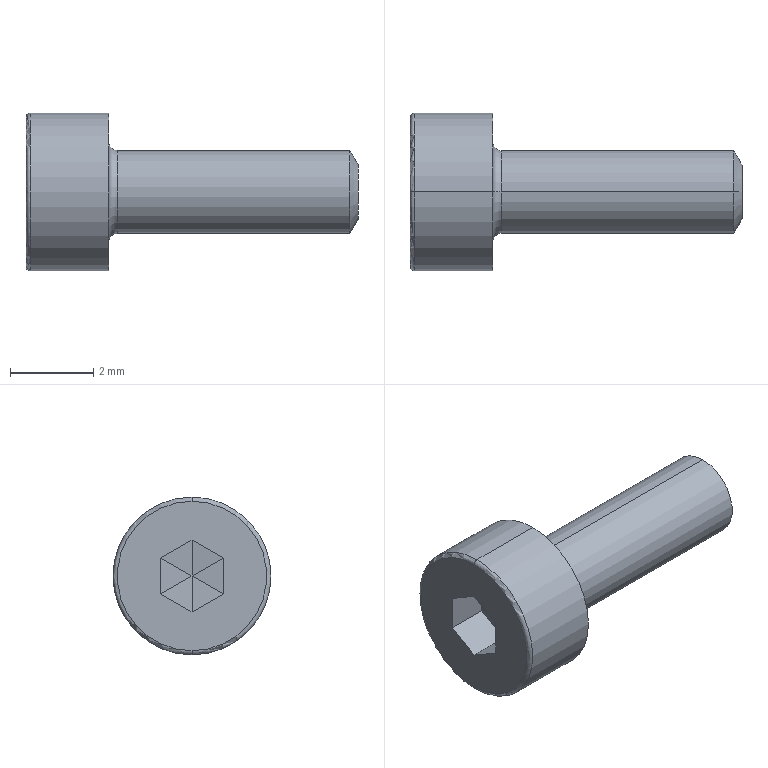Part | SolidWorks | features BlendCut 1, Cut 1, Fillet 1, LPattern 1, RevCut 1, Revolution 1 | 1 solid | 25 faces | box 8 x 3.8 x 3.8 mm | volume 39.383 mm3 | plane 15 | torus 4 | cylinder 4 | cone 2 | commonest cylinder face diameters 2 x2 3.8 x2
STEP:
#1=CARTESIAN_POINT('',(0.,0.,1.8));
#2=VERTEX_POINT('',#1);
#3=CARTESIAN_POINT('',(0.,0.,-1.8));
#4=VERTEX_POINT('',#3);
#5=CARTESIAN_POINT('',(0.,0.,0.));
#6=DIRECTION('',(-1.,0.,0.));
#7=DIRECTION('',(0.,0.,-1.));
#8=AXIS2_PLACEMENT_3D('',#5,#6,#7);
#9=CIRCLE('',#8,1.8);
#10=EDGE_CURVE('',#2,#4,#9,.T.);
#11=ORIENTED_EDGE('',*,*,#10,.F.);
#12=CARTESIAN_POINT('',(0.1,0.,1.9));
#13=VERTEX_POINT('',#12);
#14=CARTESIAN_POINT('',(0.1,0.,1.8));
#15=DIRECTION('',(0.,1.,0.));
#16=DIRECTION('',(0.,0.,1.));
#17=AXIS2_PLACEMENT_3D('',#14,#15,#16);
#18=CIRCLE('',#17,0.1);
#19=EDGE_CURVE('',#2,#13,#18,.T.);
#20=ORIENTED_EDGE('',*,*,#19,.T.);
#21=CARTESIAN_POINT('',(0.1,0.,-1.9));
#22=VERTEX_POINT('',#21);
#23=CARTESIAN_POINT('',(0.1,0.,0.));
#24=DIRECTION('',(1.,0.,0.));
#25=DIRECTION('',(0.,0.,-1.));
#26=AXIS2_PLACEMENT_3D('',#23,#24,#25);
#27=CIRCLE('',#26,1.9);
#28=EDGE_CURVE('',#22,#13,#27,.T.);
#29=ORIENTED_EDGE('',*,*,#28,.F.);
#30=CARTESIAN_POINT('',(0.1,0.,-1.8));
#31=DIRECTION('',(0.,-1.,0.));
#32=DIRECTION('',(0.,0.,-1.));
#33=AXIS2_PLACEMENT_3D('',#30,#31,#32);
#34=CIRCLE('',#33,0.1);
#35=EDGE_CURVE('',#4,#22,#34,.T.);
#36=ORIENTED_EDGE('',*,*,#35,.F.);
#37=EDGE_LOOP('',(#11,#20,#29,#36));
#38=FACE_OUTER_BOUND('',#37,.T.);
#39=CARTESIAN_POINT('',(0.1,0.,0.));
#40=DIRECTION('',(1.,0.,0.));
#41=DIRECTION('',(0.,0.,-1.));
#42=AXIS2_PLACEMENT_3D('',#39,#40,#41);
#43=TOROIDAL_SURFACE('',#42,1.8,0.1);
#44=ADVANCED_FACE('',(#38),#43,.T.);
#45=CARTESIAN_POINT('',(8.,0.,0.6536));
#46=VERTEX_POINT('',#45);
#47=CARTESIAN_POINT('',(8.,0.,-0.6536));
#48=VERTEX_POINT('',#47);
#49=CARTESIAN_POINT('',(8.,0.,0.));
#50=DIRECTION('',(-1.,0.,0.));
#51=DIRECTION('',(0.,0.,1.));
#52=AXIS2_PLACEMENT_3D('',#49,#50,#51);
#53=CIRCLE('',#52,0.6536);
#54=EDGE_CURVE('',#46,#48,#53,.T.);
#55=ORIENTED_EDGE('',*,*,#54,.T.);
#56=CARTESIAN_POINT('',(7.8,0.,-1.));
#57=VERTEX_POINT('',#56);
#58=CARTESIAN_POINT('',(7.8,0.,-1.));
#59=DIRECTION('',(-0.5,0.,-0.866));
#60=VECTOR('',#59,1000.);
#61=LINE('',#58,#60);
#62=EDGE_CURVE('',#48,#57,#61,.T.);
#63=ORIENTED_EDGE('',*,*,#62,.T.);
#64=CARTESIAN_POINT('',(7.8,0.,1.));
#65=VERTEX_POINT('',#64);
#66=CARTESIAN_POINT('',(7.8,0.,0.));
#67=DIRECTION('',(-1.,0.,0.));
#68=DIRECTION('',(0.,0.,1.));
#69=AXIS2_PLACEMENT_3D('',#66,#67,#68);
#70=CIRCLE('',#69,1.);
#71=EDGE_CURVE('',#65,#57,#70,.T.);
#72=ORIENTED_EDGE('',*,*,#71,.F.);
#73=CARTESIAN_POINT('',(7.8,0.,1.));
#74=DIRECTION('',(-0.5,0.,0.866));
#75=VECTOR('',#74,1000.);
#76=LINE('',#73,#75);
#77=EDGE_CURVE('',#46,#65,#76,.T.);
#78=ORIENTED_EDGE('',*,*,#77,.F.);
#79=EDGE_LOOP('',(#55,#63,#72,#78));
#80=FACE_OUTER_BOUND('',#79,.T.);
#81=CARTESIAN_POINT('',(7.8,0.,0.));
#82=DIRECTION('',(-1.,0.,0.));
#83=DIRECTION('',(0.,0.,1.));
#84=AXIS2_PLACEMENT_3D('',#81,#82,#83);
#85=CONICAL_SURFACE('',#84,1.,1.047);
#86=ADVANCED_FACE('',(#80),#85,.T.);
#87=CARTESIAN_POINT('',(2.,0.,-1.2));
#88=VERTEX_POINT('',#87);
#89=CARTESIAN_POINT('',(2.,0.,1.2));
#90=VERTEX_POINT('',#89);
#91=CARTESIAN_POINT('',(2.,0.,0.));
#92=DIRECTION('',(-1.,0.,0.));
#93=DIRECTION('',(0.,0.,1.));
#94=AXIS2_PLACEMENT_3D('',#91,#92,#93);
#95=CIRCLE('',#94,1.2);
#96=EDGE_CURVE('',#88,#90,#95,.T.);
#97=ORIENTED_EDGE('',*,*,#96,.F.);
#98=CARTESIAN_POINT('',(2.2,0.,-1.));
#99=VERTEX_POINT('',#98);
#100=CARTESIAN_POINT('',(2.2,0.,-1.2));
#101=DIRECTION('',(0.,1.,0.));
#102=DIRECTION('',(0.,0.,1.));
#103=AXIS2_PLACEMENT_3D('',#100,#101,#102);
#104=CIRCLE('',#103,0.2);
#105=EDGE_CURVE('',#88,#99,#104,.T.);
#106=ORIENTED_EDGE('',*,*,#105,.T.);
#107=CARTESIAN_POINT('',(2.2,0.,1.));
#108=VERTEX_POINT('',#107);
#109=CARTESIAN_POINT('',(2.2,0.,0.));
#110=DIRECTION('',(-1.,0.,0.));
#111=DIRECTION('',(0.,0.,1.));
#112=AXIS2_PLACEMENT_3D('',#109,#110,#111);
#113=CIRCLE('',#112,1.);
#114=EDGE_CURVE('',#99,#108,#113,.T.);
#115=ORIENTED_EDGE('',*,*,#114,.T.);
#116=CARTESIAN_POINT('',(2.2,0.,1.2));
#117=DIRECTION('',(0.,-1.,0.));
#118=DIRECTION('',(0.,0.,-1.));
#119=AXIS2_PLACEMENT_3D('',#116,#117,#118);
#120=CIRCLE('',#119,0.2);
#121=EDGE_CURVE('',#90,#108,#120,.T.);
#122=ORIENTED_EDGE('',*,*,#121,.F.);
#123=EDGE_LOOP('',(#97,#106,#115,#122));
#124=FACE_OUTER_BOUND('',#123,.T.);
#125=CARTESIAN_POINT('',(2.2,0.,0.));
#126=DIRECTION('',(-1.,0.,0.));
#127=DIRECTION('',(0.,0.,1.));
#128=AXIS2_PLACEMENT_3D('',#125,#126,#127);
#129=TOROIDAL_SURFACE('',#128,1.2,0.2);
#130=ADVANCED_FACE('',(#124),#129,.F.);
#131=CARTESIAN_POINT('',(2.,0.,1.9));
#132=VERTEX_POINT('',#131);
#133=CARTESIAN_POINT('',(2.,0.,-1.9));
#134=VERTEX_POINT('',#133);
#135=CARTESIAN_POINT('',(2.,0.,0.));
#136=DIRECTION('',(-1.,0.,0.));
#137=DIRECTION('',(0.,0.,1.));
#138=AXIS2_PLACEMENT_3D('',#135,#136,#137);
#139=CIRCLE('',#138,1.9);
#140=EDGE_CURVE('',#132,#134,#139,.T.);
#141=ORIENTED_EDGE('',*,*,#140,.T.);
#142=CARTESIAN_POINT('',(0.,0.,-1.9));
#143=DIRECTION('',(-1.,0.,0.));
#144=VECTOR('',#143,1000.);
#145=LINE('',#142,#144);
#146=EDGE_CURVE('',#134,#22,#145,.T.);
#147=ORIENTED_EDGE('',*,*,#146,.T.);
#148=ORIENTED_EDGE('',*,*,#28,.T.);
#149=CARTESIAN_POINT('',(0.,0.,1.9));
#150=DIRECTION('',(-1.,0.,0.));
#151=VECTOR('',#150,1000.);
#152=LINE('',#149,#151);
#153=EDGE_CURVE('',#132,#13,#152,.T.);
#154=ORIENTED_EDGE('',*,*,#153,.F.);
#155=EDGE_LOOP('',(#141,#147,#148,#154));
#156=FACE_OUTER_BOUND('',#155,.T.);
#157=CARTESIAN_POINT('',(0.,0.,0.));
#158=DIRECTION('',(-1.,0.,0.));
#159=DIRECTION('',(0.,0.,1.));
#160=AXIS2_PLACEMENT_3D('',#157,#158,#159);
#161=CYLINDRICAL_SURFACE('',#160,1.9);
#162=ADVANCED_FACE('',(#156),#161,.T.);
#163=ORIENTED_EDGE('',*,*,#71,.T.);
#164=CARTESIAN_POINT('',(0.,0.,-1.));
#165=DIRECTION('',(-1.,0.,0.));
#166=VECTOR('',#165,1000.);
#167=LINE('',#164,#166);
#168=EDGE_CURVE('',#57,#99,#167,.T.);
#169=ORIENTED_EDGE('',*,*,#168,.T.);
#170=CARTESIAN_POINT('',(2.2,0.,0.));
#171=DIRECTION('',(-1.,0.,0.));
#172=DIRECTION('',(0.,0.,1.));
#173=AXIS2_PLACEMENT_3D('',#170,#171,#172);
#174=CIRCLE('',#173,1.);
#175=EDGE_CURVE('',#108,#99,#174,.T.);
#176=ORIENTED_EDGE('',*,*,#175,.F.);
#177=CARTESIAN_POINT('',(0.,0.,1.));
#178=DIRECTION('',(-1.,0.,0.));
#179=VECTOR('',#178,1000.);
#180=LINE('',#177,#179);
#181=EDGE_CURVE('',#65,#108,#180,.T.);
#182=ORIENTED_EDGE('',*,*,#181,.F.);
#183=EDGE_LOOP('',(#163,#169,#176,#182));
#184=FACE_OUTER_BOUND('',#183,.T.);
#185=CARTESIAN_POINT('',(0.,0.,0.));
#186=DIRECTION('',(-1.,0.,0.));
#187=DIRECTION('',(0.,0.,1.));
#188=AXIS2_PLACEMENT_3D('',#185,#186,#187);
#189=CYLINDRICAL_SURFACE('',#188,1.);
#190=ADVANCED_FACE('',(#184),#189,.T.);
#191=ORIENTED_EDGE('',*,*,#168,.F.);
#192=CARTESIAN_POINT('',(7.8,0.,0.));
#193=DIRECTION('',(-1.,0.,0.));
#194=DIRECTION('',(0.,0.,1.));
#195=AXIS2_PLACEMENT_3D('',#192,#193,#194);
#196=CIRCLE('',#195,1.);
#197=EDGE_CURVE('',#57,#65,#196,.T.);
#198=ORIENTED_EDGE('',*,*,#197,.T.);
#199=ORIENTED_EDGE('',*,*,#181,.T.);
#200=ORIENTED_EDGE('',*,*,#114,.F.);
#201=EDGE_LOOP('',(#191,#198,#199,#200));
#202=FACE_OUTER_BOUND('',#201,.T.);
#203=CARTESIAN_POINT('',(0.,0.,0.));
#204=DIRECTION('',(-1.,0.,0.));
#205=DIRECTION('',(0.,0.,1.));
#206=AXIS2_PLACEMENT_3D('',#203,#204,#205);
#207=CYLINDRICAL_SURFACE('',#206,1.);
#208=ADVANCED_FACE('',(#202),#207,.T.);
#209=CARTESIAN_POINT('',(0.,0.,0.));
#210=DIRECTION('',(-1.,0.,0.));
#211=DIRECTION('',(0.,0.,-1.));
#212=AXIS2_PLACEMENT_3D('',#209,#210,#211);
#213=CIRCLE('',#212,1.8);
#214=EDGE_CURVE('',#4,#2,#213,.T.);
#215=ORIENTED_EDGE('',*,*,#214,.T.);
#216=ORIENTED_EDGE('',*,*,#10,.T.);
#217=EDGE_LOOP('',(#215,#216));
#218=FACE_OUTER_BOUND('',#217,.T.);
#219=CARTESIAN_POINT('',(0.,0.,0.865));
#220=VERTEX_POINT('',#219);
#221=CARTESIAN_POINT('',(0.,0.7491,0.4325));
#222=VERTEX_POINT('',#221);
#223=CARTESIAN_POINT('',(0.,0.,0.865));
#224=DIRECTION('',(0.,0.866,-0.5));
#225=VECTOR('',#224,1000.);
#226=LINE('',#223,#225);
#227=EDGE_CURVE('',#220,#222,#226,.T.);
#228=ORIENTED_EDGE('',*,*,#227,.F.);
#229=CARTESIAN_POINT('',(0.,-0.7491,0.4325));
#230=VERTEX_POINT('',#229);
#231=CARTESIAN_POINT('',(0.,-0.7491,0.4325));
#232=DIRECTION('',(0.,0.866,0.5));
#233=VECTOR('',#232,1000.);
#234=LINE('',#231,#233);
#235=EDGE_CURVE('',#230,#220,#234,.T.);
#236=ORIENTED_EDGE('',*,*,#235,.F.);
#237=CARTESIAN_POINT('',(0.,-0.7491,-0.4325));
#238=VERTEX_POINT('',#237);
#239=CARTESIAN_POINT('',(0.,-0.7491,-0.4325));
#240=DIRECTION('',(0.,0.,1.));
#241=VECTOR('',#240,1000.);
#242=LINE('',#239,#241);
#243=EDGE_CURVE('',#238,#230,#242,.T.);
#244=ORIENTED_EDGE('',*,*,#243,.F.);
#245=CARTESIAN_POINT('',(0.,0.,-0.865));
#246=VERTEX_POINT('',#245);
#247=CARTESIAN_POINT('',(0.,0.,-0.865));
#248=DIRECTION('',(0.,-0.866,0.5));
#249=VECTOR('',#248,1000.);
#250=LINE('',#247,#249);
#251=EDGE_CURVE('',#246,#238,#250,.T.);
#252=ORIENTED_EDGE('',*,*,#251,.F.);
#253=CARTESIAN_POINT('',(0.,0.7491,-0.4325));
#254=VERTEX_POINT('',#253);
#255=CARTESIAN_POINT('',(0.,0.7491,-0.4325));
#256=DIRECTION('',(0.,-0.866,-0.5));
#257=VECTOR('',#256,1000.);
#258=LINE('',#255,#257);
#259=EDGE_CURVE('',#254,#246,#258,.T.);
#260=ORIENTED_EDGE('',*,*,#259,.F.);
#261=CARTESIAN_POINT('',(0.,0.7491,0.4325));
#262=DIRECTION('',(0.,0.,-1.));
#263=VECTOR('',#262,1000.);
#264=LINE('',#261,#263);
#265=EDGE_CURVE('',#222,#254,#264,.T.);
#266=ORIENTED_EDGE('',*,*,#265,.F.);
#267=EDGE_LOOP('',(#228,#236,#244,#252,#260,#266));
#268=FACE_BOUND('',#267,.T.);
#269=CARTESIAN_POINT('',(0.,0.,0.));
#270=DIRECTION('',(1.,0.,0.));
#271=DIRECTION('',(0.,0.,-1.));
#272=AXIS2_PLACEMENT_3D('',#269,#270,#271);
#273=PLANE('',#272);
#274=ADVANCED_FACE('',(#218,#268),#273,.F.);
#275=ORIENTED_EDGE('',*,*,#146,.F.);
#276=CARTESIAN_POINT('',(2.,0.,0.));
#277=DIRECTION('',(-1.,0.,0.));
#278=DIRECTION('',(0.,0.,1.));
#279=AXIS2_PLACEMENT_3D('',#276,#277,#278);
#280=CIRCLE('',#279,1.9);
#281=EDGE_CURVE('',#134,#132,#280,.T.);
#282=ORIENTED_EDGE('',*,*,#281,.T.);
#283=ORIENTED_EDGE('',*,*,#153,.T.);
#284=CARTESIAN_POINT('',(0.1,0.,0.));
#285=DIRECTION('',(1.,0.,0.));
#286=DIRECTION('',(0.,0.,-1.));
#287=AXIS2_PLACEMENT_3D('',#284,#285,#286);
#288=CIRCLE('',#287,1.9);
#289=EDGE_CURVE('',#13,#22,#288,.T.);
#290=ORIENTED_EDGE('',*,*,#289,.T.);
#291=EDGE_LOOP('',(#275,#282,#283,#290));
#292=FACE_OUTER_BOUND('',#291,.T.);
#293=CARTESIAN_POINT('',(0.,0.,0.));
#294=DIRECTION('',(-1.,0.,0.));
#295=DIRECTION('',(0.,0.,1.));
#296=AXIS2_PLACEMENT_3D('',#293,#294,#295);
#297=CYLINDRICAL_SURFACE('',#296,1.9);
#298=ADVANCED_FACE('',(#292),#297,.T.);
#299=ORIENTED_EDGE('',*,*,#140,.F.);
#300=ORIENTED_EDGE('',*,*,#281,.F.);
#301=EDGE_LOOP('',(#299,#300));
#302=FACE_OUTER_BOUND('',#301,.T.);
#303=CARTESIAN_POINT('',(2.,0.,0.));
#304=DIRECTION('',(-1.,0.,0.));
#305=DIRECTION('',(0.,0.,1.));
#306=AXIS2_PLACEMENT_3D('',#303,#304,#305);
#307=CIRCLE('',#306,1.2);
#308=EDGE_CURVE('',#90,#88,#307,.T.);
#309=ORIENTED_EDGE('',*,*,#308,.T.);
#310=ORIENTED_EDGE('',*,*,#96,.T.);
#311=EDGE_LOOP('',(#309,#310));
#312=FACE_BOUND('',#311,.T.);
#313=CARTESIAN_POINT('',(2.,1.9,0.));
#314=DIRECTION('',(-1.,0.,0.));
#315=DIRECTION('',(0.,0.,1.));
#316=AXIS2_PLACEMENT_3D('',#313,#314,#315);
#317=PLANE('',#316);
#318=ADVANCED_FACE('',(#302,#312),#317,.F.);
#319=ORIENTED_EDGE('',*,*,#105,.F.);
#320=ORIENTED_EDGE('',*,*,#308,.F.);
#321=ORIENTED_EDGE('',*,*,#121,.T.);
#322=ORIENTED_EDGE('',*,*,#175,.T.);
#323=EDGE_LOOP('',(#319,#320,#321,#322));
#324=FACE_OUTER_BOUND('',#323,.T.);
#325=CARTESIAN_POINT('',(2.2,0.,0.));
#326=DIRECTION('',(-1.,0.,0.));
#327=DIRECTION('',(0.,0.,1.));
#328=AXIS2_PLACEMENT_3D('',#325,#326,#327);
#329=TOROIDAL_SURFACE('',#328,1.2,0.2);
#330=ADVANCED_FACE('',(#324),#329,.F.);
#331=ORIENTED_EDGE('',*,*,#235,.T.);
#332=CARTESIAN_POINT('',(1.,0.,0.865));
#333=VERTEX_POINT('',#332);
#334=CARTESIAN_POINT('',(1.,0.,0.865));
#335=DIRECTION('',(-1.,0.,0.));
#336=VECTOR('',#335,1000.);
#337=LINE('',#334,#336);
#338=EDGE_CURVE('',#333,#220,#337,.T.);
#339=ORIENTED_EDGE('',*,*,#338,.F.);
#340=CARTESIAN_POINT('',(1.,-0.7491,0.4325));
#341=VERTEX_POINT('',#340);
#342=CARTESIAN_POINT('',(1.,-0.7491,0.4325));
#343=DIRECTION('',(0.,0.866,0.5));
#344=VECTOR('',#343,1000.);
#345=LINE('',#342,#344);
#346=EDGE_CURVE('',#341,#333,#345,.T.);
#347=ORIENTED_EDGE('',*,*,#346,.F.);
#348=CARTESIAN_POINT('',(1.,-0.7491,0.4325));
#349=DIRECTION('',(-1.,0.,0.));
#350=VECTOR('',#349,1000.);
#351=LINE('',#348,#350);
#352=EDGE_CURVE('',#341,#230,#351,.T.);
#353=ORIENTED_EDGE('',*,*,#352,.T.);
#354=EDGE_LOOP('',(#331,#339,#347,#353));
#355=FACE_OUTER_BOUND('',#354,.T.);
#356=CARTESIAN_POINT('',(1.,-0.7491,0.4325));
#357=DIRECTION('',(0.,-0.5,0.866));
#358=DIRECTION('',(0.,-0.866,-0.5));
#359=AXIS2_PLACEMENT_3D('',#356,#357,#358);
#360=PLANE('',#359);
#361=ADVANCED_FACE('',(#355),#360,.F.);
#362=ORIENTED_EDGE('',*,*,#243,.T.);
#363=ORIENTED_EDGE('',*,*,#352,.F.);
#364=CARTESIAN_POINT('',(1.,-0.7491,-0.4325));
#365=VERTEX_POINT('',#364);
#366=CARTESIAN_POINT('',(1.,-0.7491,-0.4325));
#367=DIRECTION('',(0.,0.,1.));
#368=VECTOR('',#367,1000.);
#369=LINE('',#366,#368);
#370=EDGE_CURVE('',#365,#341,#369,.T.);
#371=ORIENTED_EDGE('',*,*,#370,.F.);
#372=CARTESIAN_POINT('',(1.,-0.7491,-0.4325));
#373=DIRECTION('',(-1.,0.,0.));
#374=VECTOR('',#373,1000.);
#375=LINE('',#372,#374);
#376=EDGE_CURVE('',#365,#238,#375,.T.);
#377=ORIENTED_EDGE('',*,*,#376,.T.);
#378=EDGE_LOOP('',(#362,#363,#371,#377));
#379=FACE_OUTER_BOUND('',#378,.T.);
#380=CARTESIAN_POINT('',(1.,-0.7491,-0.4325));
#381=DIRECTION('',(0.,-1.,0.));
#382=DIRECTION('',(0.,0.,-1.));
#383=AXIS2_PLACEMENT_3D('',#380,#381,#382);
#384=PLANE('',#383);
#385=ADVANCED_FACE('',(#379),#384,.F.);
#386=ORIENTED_EDGE('',*,*,#251,.T.);
#387=ORIENTED_EDGE('',*,*,#376,.F.);
#388=CARTESIAN_POINT('',(1.,0.,-0.865));
#389=VERTEX_POINT('',#388);
#390=CARTESIAN_POINT('',(1.,0.,-0.865));
#391=DIRECTION('',(0.,-0.866,0.5));
#392=VECTOR('',#391,1000.);
#393=LINE('',#390,#392);
#394=EDGE_CURVE('',#389,#365,#393,.T.);
#395=ORIENTED_EDGE('',*,*,#394,.F.);
#396=CARTESIAN_POINT('',(1.,0.,-0.865));
#397=DIRECTION('',(-1.,0.,0.));
#398=VECTOR('',#397,1000.);
#399=LINE('',#396,#398);
#400=EDGE_CURVE('',#389,#246,#399,.T.);
#401=ORIENTED_EDGE('',*,*,#400,.T.);
#402=EDGE_LOOP('',(#386,#387,#395,#401));
#403=FACE_OUTER_BOUND('',#402,.T.);
#404=CARTESIAN_POINT('',(1.,0.,-0.865));
#405=DIRECTION('',(0.,-0.5,-0.866));
#406=DIRECTION('',(0.,0.866,-0.5));
#407=AXIS2_PLACEMENT_3D('',#404,#405,#406);
#408=PLANE('',#407);
#409=ADVANCED_FACE('',(#403),#408,.F.);
#410=ORIENTED_EDGE('',*,*,#259,.T.);
#411=ORIENTED_EDGE('',*,*,#400,.F.);
#412=CARTESIAN_POINT('',(1.,0.7491,-0.4325));
#413=VERTEX_POINT('',#412);
#414=CARTESIAN_POINT('',(1.,0.7491,-0.4325));
#415=DIRECTION('',(0.,-0.866,-0.5));
#416=VECTOR('',#415,1000.);
#417=LINE('',#414,#416);
#418=EDGE_CURVE('',#413,#389,#417,.T.);
#419=ORIENTED_EDGE('',*,*,#418,.F.);
#420=CARTESIAN_POINT('',(1.,0.7491,-0.4325));
#421=DIRECTION('',(-1.,0.,0.));
#422=VECTOR('',#421,1000.);
#423=LINE('',#420,#422);
#424=EDGE_CURVE('',#413,#254,#423,.T.);
#425=ORIENTED_EDGE('',*,*,#424,.T.);
#426=EDGE_LOOP('',(#410,#411,#419,#425));
#427=FACE_OUTER_BOUND('',#426,.T.);
#428=CARTESIAN_POINT('',(1.,0.7491,-0.4325));
#429=DIRECTION('',(0.,0.5,-0.866));
#430=DIRECTION('',(0.,0.866,0.5));
#431=AXIS2_PLACEMENT_3D('',#428,#429,#430);
#432=PLANE('',#431);
#433=ADVANCED_FACE('',(#427),#432,.F.);
#434=ORIENTED_EDGE('',*,*,#265,.T.);
#435=ORIENTED_EDGE('',*,*,#424,.F.);
#436=CARTESIAN_POINT('',(1.,0.7491,0.4325));
#437=VERTEX_POINT('',#436);
#438=CARTESIAN_POINT('',(1.,0.7491,0.4325));
#439=DIRECTION('',(0.,0.,-1.));
#440=VECTOR('',#439,1000.);
#441=LINE('',#438,#440);
#442=EDGE_CURVE('',#437,#413,#441,.T.);
#443=ORIENTED_EDGE('',*,*,#442,.F.);
#444=CARTESIAN_POINT('',(1.,0.7491,0.4325));
#445=DIRECTION('',(-1.,0.,0.));
#446=VECTOR('',#445,1000.);
#447=LINE('',#444,#446);
#448=EDGE_CURVE('',#437,#222,#447,.T.);
#449=ORIENTED_EDGE('',*,*,#448,.T.);
#450=EDGE_LOOP('',(#434,#435,#443,#449));
#451=FACE_OUTER_BOUND('',#450,.T.);
#452=CARTESIAN_POINT('',(1.,0.7491,0.4325));
#453=DIRECTION('',(0.,1.,0.));
#454=DIRECTION('',(0.,0.,1.));
#455=AXIS2_PLACEMENT_3D('',#452,#453,#454);
#456=PLANE('',#455);
#457=ADVANCED_FACE('',(#451),#456,.F.);
#458=ORIENTED_EDGE('',*,*,#227,.T.);
#459=ORIENTED_EDGE('',*,*,#448,.F.);
#460=CARTESIAN_POINT('',(1.,0.,0.865));
#461=DIRECTION('',(0.,0.866,-0.5));
#462=VECTOR('',#461,1000.);
#463=LINE('',#460,#462);
#464=EDGE_CURVE('',#333,#437,#463,.T.);
#465=ORIENTED_EDGE('',*,*,#464,.F.);
#466=ORIENTED_EDGE('',*,*,#338,.T.);
#467=EDGE_LOOP('',(#458,#459,#465,#466));
#468=FACE_OUTER_BOUND('',#467,.T.);
#469=CARTESIAN_POINT('',(1.,0.,0.865));
#470=DIRECTION('',(0.,0.5,0.866));
#471=DIRECTION('',(0.,-0.866,0.5));
#472=AXIS2_PLACEMENT_3D('',#469,#470,#471);
#473=PLANE('',#472);
#474=ADVANCED_FACE('',(#468),#473,.F.);
#475=CARTESIAN_POINT('',(1.067,0.,0.));
#476=VERTEX_POINT('',#475);
#477=CARTESIAN_POINT('',(1.067,0.,0.));
#478=DIRECTION('',(-0.07711,-0.8634,-0.4985));
#479=VECTOR('',#478,1000.);
#480=LINE('',#477,#479);
#481=EDGE_CURVE('',#476,#365,#480,.T.);
#482=ORIENTED_EDGE('',*,*,#481,.F.);
#483=CARTESIAN_POINT('',(1.067,0.,0.));
#484=DIRECTION('',(-0.07711,0.,-0.997));
#485=VECTOR('',#484,1000.);
#486=LINE('',#483,#485);
#487=EDGE_CURVE('',#476,#389,#486,.T.);
#488=ORIENTED_EDGE('',*,*,#487,.T.);
#489=ORIENTED_EDGE('',*,*,#394,.T.);
#490=EDGE_LOOP('',(#482,#488,#489));
#491=FACE_OUTER_BOUND('',#490,.T.);
#492=CARTESIAN_POINT('',(1.,-0.7491,-0.4325));
#493=DIRECTION('',(-0.996,0.04448,0.07704));
#494=DIRECTION('',(0.07711,0.,0.997));
#495=AXIS2_PLACEMENT_3D('',#492,#493,#494);
#496=PLANE('',#495);
#497=ADVANCED_FACE('',(#491),#496,.T.);
#498=ORIENTED_EDGE('',*,*,#487,.F.);
#499=CARTESIAN_POINT('',(1.067,0.,0.));
#500=DIRECTION('',(-0.07711,0.8634,-0.4985));
#501=VECTOR('',#500,1000.);
#502=LINE('',#499,#501);
#503=EDGE_CURVE('',#476,#413,#502,.T.);
#504=ORIENTED_EDGE('',*,*,#503,.T.);
#505=ORIENTED_EDGE('',*,*,#418,.T.);
#506=EDGE_LOOP('',(#498,#504,#505));
#507=FACE_OUTER_BOUND('',#506,.T.);
#508=CARTESIAN_POINT('',(1.,0.,-0.865));
#509=DIRECTION('',(-0.996,-0.04448,0.07704));
#510=DIRECTION('',(0.07711,0.,0.997));
#511=AXIS2_PLACEMENT_3D('',#508,#509,#510);
#512=PLANE('',#511);
#513=ADVANCED_FACE('',(#507),#512,.T.);
#514=CARTESIAN_POINT('',(1.067,0.,0.));
#515=DIRECTION('',(-0.07711,-0.8634,0.4985));
#516=VECTOR('',#515,1000.);
#517=LINE('',#514,#516);
#518=EDGE_CURVE('',#476,#341,#517,.T.);
#519=ORIENTED_EDGE('',*,*,#518,.F.);
#520=ORIENTED_EDGE('',*,*,#481,.T.);
#521=ORIENTED_EDGE('',*,*,#370,.T.);
#522=EDGE_LOOP('',(#519,#520,#521));
#523=FACE_OUTER_BOUND('',#522,.T.);
#524=CARTESIAN_POINT('',(1.,-0.7491,0.4325));
#525=DIRECTION('',(-0.996,0.08895,0.));
#526=DIRECTION('',(-0.08895,-0.996,0.));
#527=AXIS2_PLACEMENT_3D('',#524,#525,#526);
#528=PLANE('',#527);
#529=ADVANCED_FACE('',(#523),#528,.T.);
#530=ORIENTED_EDGE('',*,*,#503,.F.);
#531=CARTESIAN_POINT('',(1.067,0.,0.));
#532=DIRECTION('',(-0.07711,0.8634,0.4985));
#533=VECTOR('',#532,1000.);
#534=LINE('',#531,#533);
#535=EDGE_CURVE('',#476,#437,#534,.T.);
#536=ORIENTED_EDGE('',*,*,#535,.T.);
#537=ORIENTED_EDGE('',*,*,#442,.T.);
#538=EDGE_LOOP('',(#530,#536,#537));
#539=FACE_OUTER_BOUND('',#538,.T.);
#540=CARTESIAN_POINT('',(1.,0.7491,-0.4325));
#541=DIRECTION('',(-0.996,-0.08895,0.));
#542=DIRECTION('',(0.08895,-0.996,0.));
#543=AXIS2_PLACEMENT_3D('',#540,#541,#542);
#544=PLANE('',#543);
#545=ADVANCED_FACE('',(#539),#544,.T.);
#546=CARTESIAN_POINT('',(1.067,0.,0.));
#547=DIRECTION('',(-0.07711,0.,0.997));
#548=VECTOR('',#547,1000.);
#549=LINE('',#546,#548);
#550=EDGE_CURVE('',#476,#333,#549,.T.);
#551=ORIENTED_EDGE('',*,*,#550,.F.);
#552=ORIENTED_EDGE('',*,*,#518,.T.);
#553=ORIENTED_EDGE('',*,*,#346,.T.);
#554=EDGE_LOOP('',(#551,#552,#553));
#555=FACE_OUTER_BOUND('',#554,.T.);
#556=CARTESIAN_POINT('',(1.,0.,0.865));
#557=DIRECTION('',(-0.996,0.04448,-0.07704));
#558=DIRECTION('',(-0.07711,0.,0.997));
#559=AXIS2_PLACEMENT_3D('',#556,#557,#558);
#560=PLANE('',#559);
#561=ADVANCED_FACE('',(#555),#560,.T.);
#562=ORIENTED_EDGE('',*,*,#535,.F.);
#563=ORIENTED_EDGE('',*,*,#550,.T.);
#564=ORIENTED_EDGE('',*,*,#464,.T.);
#565=EDGE_LOOP('',(#562,#563,#564));
#566=FACE_OUTER_BOUND('',#565,.T.);
#567=CARTESIAN_POINT('',(1.,0.7491,0.4325));
#568=DIRECTION('',(-0.996,-0.04448,-0.07704));
#569=DIRECTION('',(-0.07711,0.,0.997));
#570=AXIS2_PLACEMENT_3D('',#567,#568,#569);
#571=PLANE('',#570);
#572=ADVANCED_FACE('',(#566),#571,.T.);
#573=ORIENTED_EDGE('',*,*,#62,.F.);
#574=CARTESIAN_POINT('',(8.,0.,0.));
#575=DIRECTION('',(-1.,0.,0.));
#576=DIRECTION('',(0.,0.,1.));
#577=AXIS2_PLACEMENT_3D('',#574,#575,#576);
#578=CIRCLE('',#577,0.6536);
#579=EDGE_CURVE('',#48,#46,#578,.T.);
#580=ORIENTED_EDGE('',*,*,#579,.T.);
#581=ORIENTED_EDGE('',*,*,#77,.T.);
#582=ORIENTED_EDGE('',*,*,#197,.F.);
#583=EDGE_LOOP('',(#573,#580,#581,#582));
#584=FACE_OUTER_BOUND('',#583,.T.);
#585=CARTESIAN_POINT('',(7.8,0.,0.));
#586=DIRECTION('',(-1.,0.,0.));
#587=DIRECTION('',(0.,0.,1.));
#588=AXIS2_PLACEMENT_3D('',#585,#586,#587);
#589=CONICAL_SURFACE('',#588,1.,1.047);
#590=ADVANCED_FACE('',(#584),#589,.T.);
#591=ORIENTED_EDGE('',*,*,#54,.F.);
#592=ORIENTED_EDGE('',*,*,#579,.F.);
#593=EDGE_LOOP('',(#591,#592));
#594=FACE_OUTER_BOUND('',#593,.T.);
#595=CARTESIAN_POINT('',(8.,1.,0.));
#596=DIRECTION('',(-1.,0.,0.));
#597=DIRECTION('',(0.,0.,1.));
#598=AXIS2_PLACEMENT_3D('',#595,#596,#597);
#599=PLANE('',#598);
#600=ADVANCED_FACE('',(#594),#599,.F.);
#601=ORIENTED_EDGE('',*,*,#19,.F.);
#602=ORIENTED_EDGE('',*,*,#214,.F.);
#603=ORIENTED_EDGE('',*,*,#35,.T.);
#604=ORIENTED_EDGE('',*,*,#289,.F.);
#605=EDGE_LOOP('',(#601,#602,#603,#604));
#606=FACE_OUTER_BOUND('',#605,.T.);
#607=CARTESIAN_POINT('',(0.1,0.,0.));
#608=DIRECTION('',(1.,0.,0.));
#609=DIRECTION('',(0.,0.,-1.));
#610=AXIS2_PLACEMENT_3D('',#607,#608,#609);
#611=TOROIDAL_SURFACE('',#610,1.8,0.1);
#612=ADVANCED_FACE('',(#606),#611,.T.);
#613=CLOSED_SHELL('',(#44,#86,#130,#162,#190,#208,#274,#298,#318,#330,#361,#385,#409,#433,#457,#474,#497,#513,#529,#545,#561,#572,#590,#600,#612));
#614=MANIFOLD_SOLID_BREP('',#613);
#615=CARTESIAN_POINT('',(0.,0.,0.));
#616=DIRECTION('',(0.,0.,1.));
#617=DIRECTION('',(1.,0.,0.));
#618=AXIS2_PLACEMENT_3D('',#615,#616,#617);
#619=(LENGTH_UNIT()NAMED_UNIT(*)SI_UNIT(.MILLI.,.METRE.));
#620=UNCERTAINTY_MEASURE_WITH_UNIT(LENGTH_MEASURE(0.00001),#619,'','');
#621=(NAMED_UNIT(*)PLANE_ANGLE_UNIT()SI_UNIT($,.RADIAN.));
#622=(NAMED_UNIT(*)SI_UNIT($,.STERADIAN.)SOLID_ANGLE_UNIT());
#623=(GEOMETRIC_REPRESENTATION_CONTEXT(3)GLOBAL_UNCERTAINTY_ASSIGNED_CONTEXT((#620))GLOBAL_UNIT_ASSIGNED_CONTEXT((#619,#621,#622))REPRESENTATION_CONTEXT('',''));
#624=ADVANCED_BREP_SHAPE_REPRESENTATION('',(#614,#618),#623);